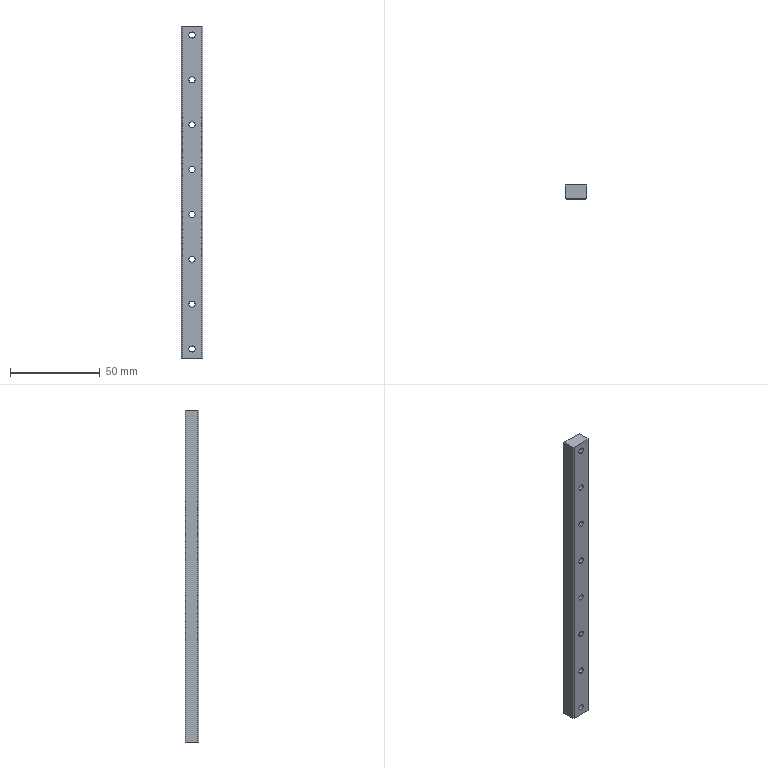Part | SolidWorks | features Chamfer 1, Extrusion 1, HoleWzd 1, LPattern 1 | 1 solid | 48 faces | box 12 x 7.5 x 185 mm | volume 15537 mm3 | cylinder 32 | plane 16 | commonest cylinder face diameters 3.4 x16 6 x16
STEP:
#1=CARTESIAN_POINT('',(0.,-3.75,178.3));
#2=VERTEX_POINT('',#1);
#3=CARTESIAN_POINT('',(0.,-3.75,181.7));
#4=VERTEX_POINT('',#3);
#5=CARTESIAN_POINT('',(0.,-3.75,180.));
#6=DIRECTION('',(0.,1.,0.));
#7=DIRECTION('',(0.,0.,1.));
#8=AXIS2_PLACEMENT_3D('',#5,#6,#7);
#9=CIRCLE('',#8,1.7);
#10=EDGE_CURVE('',#2,#4,#9,.T.);
#11=ORIENTED_EDGE('',*,*,#10,.F.);
#12=CARTESIAN_POINT('',(0.,0.35,178.3));
#13=VERTEX_POINT('',#12);
#14=CARTESIAN_POINT('',(0.,3.75,178.3));
#15=DIRECTION('',(0.,1.,0.));
#16=VECTOR('',#15,1000.);
#17=LINE('',#14,#16);
#18=EDGE_CURVE('',#2,#13,#17,.T.);
#19=ORIENTED_EDGE('',*,*,#18,.T.);
#20=CARTESIAN_POINT('',(0.,0.35,181.7));
#21=VERTEX_POINT('',#20);
#22=CARTESIAN_POINT('',(0.,0.35,180.));
#23=DIRECTION('',(0.,1.,0.));
#24=DIRECTION('',(0.,0.,1.));
#25=AXIS2_PLACEMENT_3D('',#22,#23,#24);
#26=CIRCLE('',#25,1.7);
#27=EDGE_CURVE('',#13,#21,#26,.T.);
#28=ORIENTED_EDGE('',*,*,#27,.T.);
#29=CARTESIAN_POINT('',(0.,3.75,181.7));
#30=DIRECTION('',(0.,1.,0.));
#31=VECTOR('',#30,1000.);
#32=LINE('',#29,#31);
#33=EDGE_CURVE('',#4,#21,#32,.T.);
#34=ORIENTED_EDGE('',*,*,#33,.F.);
#35=EDGE_LOOP('',(#11,#19,#28,#34));
#36=FACE_OUTER_BOUND('',#35,.T.);
#37=CARTESIAN_POINT('',(0.,3.75,180.));
#38=DIRECTION('',(0.,1.,0.));
#39=DIRECTION('',(0.,0.,1.));
#40=AXIS2_PLACEMENT_3D('',#37,#38,#39);
#41=CYLINDRICAL_SURFACE('',#40,1.7);
#42=ADVANCED_FACE('',(#36),#41,.F.);
#43=CARTESIAN_POINT('',(0.,0.35,177.));
#44=VERTEX_POINT('',#43);
#45=CARTESIAN_POINT('',(0.,0.35,183.));
#46=VERTEX_POINT('',#45);
#47=CARTESIAN_POINT('',(0.,0.35,180.));
#48=DIRECTION('',(0.,1.,0.));
#49=DIRECTION('',(0.,0.,1.));
#50=AXIS2_PLACEMENT_3D('',#47,#48,#49);
#51=CIRCLE('',#50,3.);
#52=EDGE_CURVE('',#44,#46,#51,.T.);
#53=ORIENTED_EDGE('',*,*,#52,.F.);
#54=CARTESIAN_POINT('',(0.,3.75,177.));
#55=VERTEX_POINT('',#54);
#56=CARTESIAN_POINT('',(0.,3.75,177.));
#57=DIRECTION('',(0.,1.,0.));
#58=VECTOR('',#57,1000.);
#59=LINE('',#56,#58);
#60=EDGE_CURVE('',#44,#55,#59,.T.);
#61=ORIENTED_EDGE('',*,*,#60,.T.);
#62=CARTESIAN_POINT('',(0.,3.75,183.));
#63=VERTEX_POINT('',#62);
#64=CARTESIAN_POINT('',(0.,3.75,180.));
#65=DIRECTION('',(0.,1.,0.));
#66=DIRECTION('',(0.,0.,1.));
#67=AXIS2_PLACEMENT_3D('',#64,#65,#66);
#68=CIRCLE('',#67,3.);
#69=EDGE_CURVE('',#55,#63,#68,.T.);
#70=ORIENTED_EDGE('',*,*,#69,.T.);
#71=CARTESIAN_POINT('',(0.,3.75,183.));
#72=DIRECTION('',(0.,1.,0.));
#73=VECTOR('',#72,1000.);
#74=LINE('',#71,#73);
#75=EDGE_CURVE('',#46,#63,#74,.T.);
#76=ORIENTED_EDGE('',*,*,#75,.F.);
#77=EDGE_LOOP('',(#53,#61,#70,#76));
#78=FACE_OUTER_BOUND('',#77,.T.);
#79=CARTESIAN_POINT('',(0.,3.75,180.));
#80=DIRECTION('',(0.,1.,0.));
#81=DIRECTION('',(0.,0.,1.));
#82=AXIS2_PLACEMENT_3D('',#79,#80,#81);
#83=CYLINDRICAL_SURFACE('',#82,3.);
#84=ADVANCED_FACE('',(#78),#83,.F.);
#85=CARTESIAN_POINT('',(0.,-3.75,153.3));
#86=VERTEX_POINT('',#85);
#87=CARTESIAN_POINT('',(0.,-3.75,156.7));
#88=VERTEX_POINT('',#87);
#89=CARTESIAN_POINT('',(0.,-3.75,155.));
#90=DIRECTION('',(0.,1.,0.));
#91=DIRECTION('',(0.,0.,1.));
#92=AXIS2_PLACEMENT_3D('',#89,#90,#91);
#93=CIRCLE('',#92,1.7);
#94=EDGE_CURVE('',#86,#88,#93,.T.);
#95=ORIENTED_EDGE('',*,*,#94,.F.);
#96=CARTESIAN_POINT('',(0.,0.35,153.3));
#97=VERTEX_POINT('',#96);
#98=CARTESIAN_POINT('',(0.,3.75,153.3));
#99=DIRECTION('',(0.,1.,0.));
#100=VECTOR('',#99,1000.);
#101=LINE('',#98,#100);
#102=EDGE_CURVE('',#86,#97,#101,.T.);
#103=ORIENTED_EDGE('',*,*,#102,.T.);
#104=CARTESIAN_POINT('',(0.,0.35,156.7));
#105=VERTEX_POINT('',#104);
#106=CARTESIAN_POINT('',(0.,0.35,155.));
#107=DIRECTION('',(0.,1.,0.));
#108=DIRECTION('',(0.,0.,1.));
#109=AXIS2_PLACEMENT_3D('',#106,#107,#108);
#110=CIRCLE('',#109,1.7);
#111=EDGE_CURVE('',#97,#105,#110,.T.);
#112=ORIENTED_EDGE('',*,*,#111,.T.);
#113=CARTESIAN_POINT('',(0.,3.75,156.7));
#114=DIRECTION('',(0.,1.,0.));
#115=VECTOR('',#114,1000.);
#116=LINE('',#113,#115);
#117=EDGE_CURVE('',#88,#105,#116,.T.);
#118=ORIENTED_EDGE('',*,*,#117,.F.);
#119=EDGE_LOOP('',(#95,#103,#112,#118));
#120=FACE_OUTER_BOUND('',#119,.T.);
#121=CARTESIAN_POINT('',(0.,3.75,155.));
#122=DIRECTION('',(0.,1.,0.));
#123=DIRECTION('',(0.,0.,1.));
#124=AXIS2_PLACEMENT_3D('',#121,#122,#123);
#125=CYLINDRICAL_SURFACE('',#124,1.7);
#126=ADVANCED_FACE('',(#120),#125,.F.);
#127=CARTESIAN_POINT('',(0.,0.35,152.));
#128=VERTEX_POINT('',#127);
#129=CARTESIAN_POINT('',(0.,0.35,158.));
#130=VERTEX_POINT('',#129);
#131=CARTESIAN_POINT('',(0.,0.35,155.));
#132=DIRECTION('',(0.,1.,0.));
#133=DIRECTION('',(0.,0.,1.));
#134=AXIS2_PLACEMENT_3D('',#131,#132,#133);
#135=CIRCLE('',#134,3.);
#136=EDGE_CURVE('',#128,#130,#135,.T.);
#137=ORIENTED_EDGE('',*,*,#136,.F.);
#138=CARTESIAN_POINT('',(0.,3.75,152.));
#139=VERTEX_POINT('',#138);
#140=CARTESIAN_POINT('',(0.,3.75,152.));
#141=DIRECTION('',(0.,1.,0.));
#142=VECTOR('',#141,1000.);
#143=LINE('',#140,#142);
#144=EDGE_CURVE('',#128,#139,#143,.T.);
#145=ORIENTED_EDGE('',*,*,#144,.T.);
#146=CARTESIAN_POINT('',(0.,3.75,158.));
#147=VERTEX_POINT('',#146);
#148=CARTESIAN_POINT('',(0.,3.75,155.));
#149=DIRECTION('',(0.,1.,0.));
#150=DIRECTION('',(0.,0.,1.));
#151=AXIS2_PLACEMENT_3D('',#148,#149,#150);
#152=CIRCLE('',#151,3.);
#153=EDGE_CURVE('',#139,#147,#152,.T.);
#154=ORIENTED_EDGE('',*,*,#153,.T.);
#155=CARTESIAN_POINT('',(0.,3.75,158.));
#156=DIRECTION('',(0.,1.,0.));
#157=VECTOR('',#156,1000.);
#158=LINE('',#155,#157);
#159=EDGE_CURVE('',#130,#147,#158,.T.);
#160=ORIENTED_EDGE('',*,*,#159,.F.);
#161=EDGE_LOOP('',(#137,#145,#154,#160));
#162=FACE_OUTER_BOUND('',#161,.T.);
#163=CARTESIAN_POINT('',(0.,3.75,155.));
#164=DIRECTION('',(0.,1.,0.));
#165=DIRECTION('',(0.,0.,1.));
#166=AXIS2_PLACEMENT_3D('',#163,#164,#165);
#167=CYLINDRICAL_SURFACE('',#166,3.);
#168=ADVANCED_FACE('',(#162),#167,.F.);
#169=CARTESIAN_POINT('',(0.,-3.75,128.3));
#170=VERTEX_POINT('',#169);
#171=CARTESIAN_POINT('',(0.,-3.75,131.7));
#172=VERTEX_POINT('',#171);
#173=CARTESIAN_POINT('',(0.,-3.75,130.));
#174=DIRECTION('',(0.,1.,0.));
#175=DIRECTION('',(0.,0.,1.));
#176=AXIS2_PLACEMENT_3D('',#173,#174,#175);
#177=CIRCLE('',#176,1.7);
#178=EDGE_CURVE('',#170,#172,#177,.T.);
#179=ORIENTED_EDGE('',*,*,#178,.F.);
#180=CARTESIAN_POINT('',(0.,0.35,128.3));
#181=VERTEX_POINT('',#180);
#182=CARTESIAN_POINT('',(0.,3.75,128.3));
#183=DIRECTION('',(0.,1.,0.));
#184=VECTOR('',#183,1000.);
#185=LINE('',#182,#184);
#186=EDGE_CURVE('',#170,#181,#185,.T.);
#187=ORIENTED_EDGE('',*,*,#186,.T.);
#188=CARTESIAN_POINT('',(0.,0.35,131.7));
#189=VERTEX_POINT('',#188);
#190=CARTESIAN_POINT('',(0.,0.35,130.));
#191=DIRECTION('',(0.,1.,0.));
#192=DIRECTION('',(0.,0.,1.));
#193=AXIS2_PLACEMENT_3D('',#190,#191,#192);
#194=CIRCLE('',#193,1.7);
#195=EDGE_CURVE('',#181,#189,#194,.T.);
#196=ORIENTED_EDGE('',*,*,#195,.T.);
#197=CARTESIAN_POINT('',(0.,3.75,131.7));
#198=DIRECTION('',(0.,1.,0.));
#199=VECTOR('',#198,1000.);
#200=LINE('',#197,#199);
#201=EDGE_CURVE('',#172,#189,#200,.T.);
#202=ORIENTED_EDGE('',*,*,#201,.F.);
#203=EDGE_LOOP('',(#179,#187,#196,#202));
#204=FACE_OUTER_BOUND('',#203,.T.);
#205=CARTESIAN_POINT('',(0.,3.75,130.));
#206=DIRECTION('',(0.,1.,0.));
#207=DIRECTION('',(0.,0.,1.));
#208=AXIS2_PLACEMENT_3D('',#205,#206,#207);
#209=CYLINDRICAL_SURFACE('',#208,1.7);
#210=ADVANCED_FACE('',(#204),#209,.F.);
#211=CARTESIAN_POINT('',(0.,0.35,127.));
#212=VERTEX_POINT('',#211);
#213=CARTESIAN_POINT('',(0.,0.35,133.));
#214=VERTEX_POINT('',#213);
#215=CARTESIAN_POINT('',(0.,0.35,130.));
#216=DIRECTION('',(0.,1.,0.));
#217=DIRECTION('',(0.,0.,1.));
#218=AXIS2_PLACEMENT_3D('',#215,#216,#217);
#219=CIRCLE('',#218,3.);
#220=EDGE_CURVE('',#212,#214,#219,.T.);
#221=ORIENTED_EDGE('',*,*,#220,.F.);
#222=CARTESIAN_POINT('',(0.,3.75,127.));
#223=VERTEX_POINT('',#222);
#224=CARTESIAN_POINT('',(0.,3.75,127.));
#225=DIRECTION('',(0.,1.,0.));
#226=VECTOR('',#225,1000.);
#227=LINE('',#224,#226);
#228=EDGE_CURVE('',#212,#223,#227,.T.);
#229=ORIENTED_EDGE('',*,*,#228,.T.);
#230=CARTESIAN_POINT('',(0.,3.75,133.));
#231=VERTEX_POINT('',#230);
#232=CARTESIAN_POINT('',(0.,3.75,130.));
#233=DIRECTION('',(0.,1.,0.));
#234=DIRECTION('',(0.,0.,1.));
#235=AXIS2_PLACEMENT_3D('',#232,#233,#234);
#236=CIRCLE('',#235,3.);
#237=EDGE_CURVE('',#223,#231,#236,.T.);
#238=ORIENTED_EDGE('',*,*,#237,.T.);
#239=CARTESIAN_POINT('',(0.,3.75,133.));
#240=DIRECTION('',(0.,1.,0.));
#241=VECTOR('',#240,1000.);
#242=LINE('',#239,#241);
#243=EDGE_CURVE('',#214,#231,#242,.T.);
#244=ORIENTED_EDGE('',*,*,#243,.F.);
#245=EDGE_LOOP('',(#221,#229,#238,#244));
#246=FACE_OUTER_BOUND('',#245,.T.);
#247=CARTESIAN_POINT('',(0.,3.75,130.));
#248=DIRECTION('',(0.,1.,0.));
#249=DIRECTION('',(0.,0.,1.));
#250=AXIS2_PLACEMENT_3D('',#247,#248,#249);
#251=CYLINDRICAL_SURFACE('',#250,3.);
#252=ADVANCED_FACE('',(#246),#251,.F.);
#253=CARTESIAN_POINT('',(0.,-3.75,103.3));
#254=VERTEX_POINT('',#253);
#255=CARTESIAN_POINT('',(0.,-3.75,106.7));
#256=VERTEX_POINT('',#255);
#257=CARTESIAN_POINT('',(0.,-3.75,105.));
#258=DIRECTION('',(0.,1.,0.));
#259=DIRECTION('',(0.,0.,1.));
#260=AXIS2_PLACEMENT_3D('',#257,#258,#259);
#261=CIRCLE('',#260,1.7);
#262=EDGE_CURVE('',#254,#256,#261,.T.);
#263=ORIENTED_EDGE('',*,*,#262,.F.);
#264=CARTESIAN_POINT('',(0.,0.35,103.3));
#265=VERTEX_POINT('',#264);
#266=CARTESIAN_POINT('',(0.,3.75,103.3));
#267=DIRECTION('',(0.,1.,0.));
#268=VECTOR('',#267,1000.);
#269=LINE('',#266,#268);
#270=EDGE_CURVE('',#254,#265,#269,.T.);
#271=ORIENTED_EDGE('',*,*,#270,.T.);
#272=CARTESIAN_POINT('',(0.,0.35,106.7));
#273=VERTEX_POINT('',#272);
#274=CARTESIAN_POINT('',(0.,0.35,105.));
#275=DIRECTION('',(0.,1.,0.));
#276=DIRECTION('',(0.,0.,1.));
#277=AXIS2_PLACEMENT_3D('',#274,#275,#276);
#278=CIRCLE('',#277,1.7);
#279=EDGE_CURVE('',#265,#273,#278,.T.);
#280=ORIENTED_EDGE('',*,*,#279,.T.);
#281=CARTESIAN_POINT('',(0.,3.75,106.7));
#282=DIRECTION('',(0.,1.,0.));
#283=VECTOR('',#282,1000.);
#284=LINE('',#281,#283);
#285=EDGE_CURVE('',#256,#273,#284,.T.);
#286=ORIENTED_EDGE('',*,*,#285,.F.);
#287=EDGE_LOOP('',(#263,#271,#280,#286));
#288=FACE_OUTER_BOUND('',#287,.T.);
#289=CARTESIAN_POINT('',(0.,3.75,105.));
#290=DIRECTION('',(0.,1.,0.));
#291=DIRECTION('',(0.,0.,1.));
#292=AXIS2_PLACEMENT_3D('',#289,#290,#291);
#293=CYLINDRICAL_SURFACE('',#292,1.7);
#294=ADVANCED_FACE('',(#288),#293,.F.);
#295=CARTESIAN_POINT('',(0.,0.35,102.));
#296=VERTEX_POINT('',#295);
#297=CARTESIAN_POINT('',(0.,0.35,108.));
#298=VERTEX_POINT('',#297);
#299=CARTESIAN_POINT('',(0.,0.35,105.));
#300=DIRECTION('',(0.,1.,0.));
#301=DIRECTION('',(0.,0.,1.));
#302=AXIS2_PLACEMENT_3D('',#299,#300,#301);
#303=CIRCLE('',#302,3.);
#304=EDGE_CURVE('',#296,#298,#303,.T.);
#305=ORIENTED_EDGE('',*,*,#304,.F.);
#306=CARTESIAN_POINT('',(0.,3.75,102.));
#307=VERTEX_POINT('',#306);
#308=CARTESIAN_POINT('',(0.,3.75,102.));
#309=DIRECTION('',(0.,1.,0.));
#310=VECTOR('',#309,1000.);
#311=LINE('',#308,#310);
#312=EDGE_CURVE('',#296,#307,#311,.T.);
#313=ORIENTED_EDGE('',*,*,#312,.T.);
#314=CARTESIAN_POINT('',(0.,3.75,108.));
#315=VERTEX_POINT('',#314);
#316=CARTESIAN_POINT('',(0.,3.75,105.));
#317=DIRECTION('',(0.,1.,0.));
#318=DIRECTION('',(0.,0.,1.));
#319=AXIS2_PLACEMENT_3D('',#316,#317,#318);
#320=CIRCLE('',#319,3.);
#321=EDGE_CURVE('',#307,#315,#320,.T.);
#322=ORIENTED_EDGE('',*,*,#321,.T.);
#323=CARTESIAN_POINT('',(0.,3.75,108.));
#324=DIRECTION('',(0.,1.,0.));
#325=VECTOR('',#324,1000.);
#326=LINE('',#323,#325);
#327=EDGE_CURVE('',#298,#315,#326,.T.);
#328=ORIENTED_EDGE('',*,*,#327,.F.);
#329=EDGE_LOOP('',(#305,#313,#322,#328));
#330=FACE_OUTER_BOUND('',#329,.T.);
#331=CARTESIAN_POINT('',(0.,3.75,105.));
#332=DIRECTION('',(0.,1.,0.));
#333=DIRECTION('',(0.,0.,1.));
#334=AXIS2_PLACEMENT_3D('',#331,#332,#333);
#335=CYLINDRICAL_SURFACE('',#334,3.);
#336=ADVANCED_FACE('',(#330),#335,.F.);
#337=CARTESIAN_POINT('',(0.,-3.75,78.3));
#338=VERTEX_POINT('',#337);
#339=CARTESIAN_POINT('',(0.,-3.75,81.7));
#340=VERTEX_POINT('',#339);
#341=CARTESIAN_POINT('',(0.,-3.75,80.));
#342=DIRECTION('',(0.,1.,0.));
#343=DIRECTION('',(0.,0.,1.));
#344=AXIS2_PLACEMENT_3D('',#341,#342,#343);
#345=CIRCLE('',#344,1.7);
#346=EDGE_CURVE('',#338,#340,#345,.T.);
#347=ORIENTED_EDGE('',*,*,#346,.F.);
#348=CARTESIAN_POINT('',(0.,0.35,78.3));
#349=VERTEX_POINT('',#348);
#350=CARTESIAN_POINT('',(0.,3.75,78.3));
#351=DIRECTION('',(0.,1.,0.));
#352=VECTOR('',#351,1000.);
#353=LINE('',#350,#352);
#354=EDGE_CURVE('',#338,#349,#353,.T.);
#355=ORIENTED_EDGE('',*,*,#354,.T.);
#356=CARTESIAN_POINT('',(0.,0.35,81.7));
#357=VERTEX_POINT('',#356);
#358=CARTESIAN_POINT('',(0.,0.35,80.));
#359=DIRECTION('',(0.,1.,0.));
#360=DIRECTION('',(0.,0.,1.));
#361=AXIS2_PLACEMENT_3D('',#358,#359,#360);
#362=CIRCLE('',#361,1.7);
#363=EDGE_CURVE('',#349,#357,#362,.T.);
#364=ORIENTED_EDGE('',*,*,#363,.T.);
#365=CARTESIAN_POINT('',(0.,3.75,81.7));
#366=DIRECTION('',(0.,1.,0.));
#367=VECTOR('',#366,1000.);
#368=LINE('',#365,#367);
#369=EDGE_CURVE('',#340,#357,#368,.T.);
#370=ORIENTED_EDGE('',*,*,#369,.F.);
#371=EDGE_LOOP('',(#347,#355,#364,#370));
#372=FACE_OUTER_BOUND('',#371,.T.);
#373=CARTESIAN_POINT('',(0.,3.75,80.));
#374=DIRECTION('',(0.,1.,0.));
#375=DIRECTION('',(0.,0.,1.));
#376=AXIS2_PLACEMENT_3D('',#373,#374,#375);
#377=CYLINDRICAL_SURFACE('',#376,1.7);
#378=ADVANCED_FACE('',(#372),#377,.F.);
#379=CARTESIAN_POINT('',(0.,0.35,77.));
#380=VERTEX_POINT('',#379);
#381=CARTESIAN_POINT('',(0.,0.35,83.));
#382=VERTEX_POINT('',#381);
#383=CARTESIAN_POINT('',(0.,0.35,80.));
#384=DIRECTION('',(0.,1.,0.));
#385=DIRECTION('',(0.,0.,1.));
#386=AXIS2_PLACEMENT_3D('',#383,#384,#385);
#387=CIRCLE('',#386,3.);
#388=EDGE_CURVE('',#380,#382,#387,.T.);
#389=ORIENTED_EDGE('',*,*,#388,.F.);
#390=CARTESIAN_POINT('',(0.,3.75,77.));
#391=VERTEX_POINT('',#390);
#392=CARTESIAN_POINT('',(0.,3.75,77.));
#393=DIRECTION('',(0.,1.,0.));
#394=VECTOR('',#393,1000.);
#395=LINE('',#392,#394);
#396=EDGE_CURVE('',#380,#391,#395,.T.);
#397=ORIENTED_EDGE('',*,*,#396,.T.);
#398=CARTESIAN_POINT('',(0.,3.75,83.));
#399=VERTEX_POINT('',#398);
#400=CARTESIAN_POINT('',(0.,3.75,80.));
#401=DIRECTION('',(0.,1.,0.));
#402=DIRECTION('',(0.,0.,1.));
#403=AXIS2_PLACEMENT_3D('',#400,#401,#402);
#404=CIRCLE('',#403,3.);
#405=EDGE_CURVE('',#391,#399,#404,.T.);
#406=ORIENTED_EDGE('',*,*,#405,.T.);
#407=CARTESIAN_POINT('',(0.,3.75,83.));
#408=DIRECTION('',(0.,1.,0.));
#409=VECTOR('',#408,1000.);
#410=LINE('',#407,#409);
#411=EDGE_CURVE('',#382,#399,#410,.T.);
#412=ORIENTED_EDGE('',*,*,#411,.F.);
#413=EDGE_LOOP('',(#389,#397,#406,#412));
#414=FACE_OUTER_BOUND('',#413,.T.);
#415=CARTESIAN_POINT('',(0.,3.75,80.));
#416=DIRECTION('',(0.,1.,0.));
#417=DIRECTION('',(0.,0.,1.));
#418=AXIS2_PLACEMENT_3D('',#415,#416,#417);
#419=CYLINDRICAL_SURFACE('',#418,3.);
#420=ADVANCED_FACE('',(#414),#419,.F.);
#421=CARTESIAN_POINT('',(0.,-3.75,53.3));
#422=VERTEX_POINT('',#421);
#423=CARTESIAN_POINT('',(0.,-3.75,56.7));
#424=VERTEX_POINT('',#423);
#425=CARTESIAN_POINT('',(0.,-3.75,55.));
#426=DIRECTION('',(0.,1.,0.));
#427=DIRECTION('',(0.,0.,1.));
#428=AXIS2_PLACEMENT_3D('',#425,#426,#427);
#429=CIRCLE('',#428,1.7);
#430=EDGE_CURVE('',#422,#424,#429,.T.);
#431=ORIENTED_EDGE('',*,*,#430,.F.);
#432=CARTESIAN_POINT('',(0.,0.35,53.3));
#433=VERTEX_POINT('',#432);
#434=CARTESIAN_POINT('',(0.,3.75,53.3));
#435=DIRECTION('',(0.,1.,0.));
#436=VECTOR('',#435,1000.);
#437=LINE('',#434,#436);
#438=EDGE_CURVE('',#422,#433,#437,.T.);
#439=ORIENTED_EDGE('',*,*,#438,.T.);
#440=CARTESIAN_POINT('',(0.,0.35,56.7));
#441=VERTEX_POINT('',#440);
#442=CARTESIAN_POINT('',(0.,0.35,55.));
#443=DIRECTION('',(0.,1.,0.));
#444=DIRECTION('',(0.,0.,1.));
#445=AXIS2_PLACEMENT_3D('',#442,#443,#444);
#446=CIRCLE('',#445,1.7);
#447=EDGE_CURVE('',#433,#441,#446,.T.);
#448=ORIENTED_EDGE('',*,*,#447,.T.);
#449=CARTESIAN_POINT('',(0.,3.75,56.7));
#450=DIRECTION('',(0.,1.,0.));
#451=VECTOR('',#450,1000.);
#452=LINE('',#449,#451);
#453=EDGE_CURVE('',#424,#441,#452,.T.);
#454=ORIENTED_EDGE('',*,*,#453,.F.);
#455=EDGE_LOOP('',(#431,#439,#448,#454));
#456=FACE_OUTER_BOUND('',#455,.T.);
#457=CARTESIAN_POINT('',(0.,3.75,55.));
#458=DIRECTION('',(0.,1.,0.));
#459=DIRECTION('',(0.,0.,1.));
#460=AXIS2_PLACEMENT_3D('',#457,#458,#459);
#461=CYLINDRICAL_SURFACE('',#460,1.7);
#462=ADVANCED_FACE('',(#456),#461,.F.);
#463=CARTESIAN_POINT('',(0.,0.35,52.));
#464=VERTEX_POINT('',#463);
#465=CARTESIAN_POINT('',(0.,0.35,58.));
#466=VERTEX_POINT('',#465);
#467=CARTESIAN_POINT('',(0.,0.35,55.));
#468=DIRECTION('',(0.,1.,0.));
#469=DIRECTION('',(0.,0.,1.));
#470=AXIS2_PLACEMENT_3D('',#467,#468,#469);
#471=CIRCLE('',#470,3.);
#472=EDGE_CURVE('',#464,#466,#471,.T.);
#473=ORIENTED_EDGE('',*,*,#472,.F.);
#474=CARTESIAN_POINT('',(0.,3.75,52.));
#475=VERTEX_POINT('',#474);
#476=CARTESIAN_POINT('',(0.,3.75,52.));
#477=DIRECTION('',(0.,1.,0.));
#478=VECTOR('',#477,1000.);
#479=LINE('',#476,#478);
#480=EDGE_CURVE('',#464,#475,#479,.T.);
#481=ORIENTED_EDGE('',*,*,#480,.T.);
#482=CARTESIAN_POINT('',(0.,3.75,58.));
#483=VERTEX_POINT('',#482);
#484=CARTESIAN_POINT('',(0.,3.75,55.));
#485=DIRECTION('',(0.,1.,0.));
#486=DIRECTION('',(0.,0.,1.));
#487=AXIS2_PLACEMENT_3D('',#484,#485,#486);
#488=CIRCLE('',#487,3.);
#489=EDGE_CURVE('',#475,#483,#488,.T.);
#490=ORIENTED_EDGE('',*,*,#489,.T.);
#491=CARTESIAN_POINT('',(0.,3.75,58.));
#492=DIRECTION('',(0.,1.,0.));
#493=VECTOR('',#492,1000.);
#494=LINE('',#491,#493);
#495=EDGE_CURVE('',#466,#483,#494,.T.);
#496=ORIENTED_EDGE('',*,*,#495,.F.);
#497=EDGE_LOOP('',(#473,#481,#490,#496));
#498=FACE_OUTER_BOUND('',#497,.T.);
#499=CARTESIAN_POINT('',(0.,3.75,55.));
#500=DIRECTION('',(0.,1.,0.));
#501=DIRECTION('',(0.,0.,1.));
#502=AXIS2_PLACEMENT_3D('',#499,#500,#501);
#503=CYLINDRICAL_SURFACE('',#502,3.);
#504=ADVANCED_FACE('',(#498),#503,.F.);
#505=CARTESIAN_POINT('',(0.,0.35,27.));
#506=VERTEX_POINT('',#505);
#507=CARTESIAN_POINT('',(0.,0.35,33.));
#508=VERTEX_POINT('',#507);
#509=CARTESIAN_POINT('',(0.,0.35,30.));
#510=DIRECTION('',(0.,1.,0.));
#511=DIRECTION('',(0.,0.,1.));
#512=AXIS2_PLACEMENT_3D('',#509,#510,#511);
#513=CIRCLE('',#512,3.);
#514=EDGE_CURVE('',#506,#508,#513,.T.);
#515=ORIENTED_EDGE('',*,*,#514,.F.);
#516=CARTESIAN_POINT('',(0.,3.75,27.));
#517=VERTEX_POINT('',#516);
#518=CARTESIAN_POINT('',(0.,3.75,27.));
#519=DIRECTION('',(0.,1.,0.));
#520=VECTOR('',#519,1000.);
#521=LINE('',#518,#520);
#522=EDGE_CURVE('',#506,#517,#521,.T.);
#523=ORIENTED_EDGE('',*,*,#522,.T.);
#524=CARTESIAN_POINT('',(0.,3.75,33.));
#525=VERTEX_POINT('',#524);
#526=CARTESIAN_POINT('',(0.,3.75,30.));
#527=DIRECTION('',(0.,1.,0.));
#528=DIRECTION('',(0.,0.,1.));
#529=AXIS2_PLACEMENT_3D('',#526,#527,#528);
#530=CIRCLE('',#529,3.);
#531=EDGE_CURVE('',#517,#525,#530,.T.);
#532=ORIENTED_EDGE('',*,*,#531,.T.);
#533=CARTESIAN_POINT('',(0.,3.75,33.));
#534=DIRECTION('',(0.,1.,0.));
#535=VECTOR('',#534,1000.);
#536=LINE('',#533,#535);
#537=EDGE_CURVE('',#508,#525,#536,.T.);
#538=ORIENTED_EDGE('',*,*,#537,.F.);
#539=EDGE_LOOP('',(#515,#523,#532,#538));
#540=FACE_OUTER_BOUND('',#539,.T.);
#541=CARTESIAN_POINT('',(0.,3.75,30.));
#542=DIRECTION('',(0.,1.,0.));
#543=DIRECTION('',(0.,0.,1.));
#544=AXIS2_PLACEMENT_3D('',#541,#542,#543);
#545=CYLINDRICAL_SURFACE('',#544,3.);
#546=ADVANCED_FACE('',(#540),#545,.F.);
#547=CARTESIAN_POINT('',(0.,-3.75,28.3));
#548=VERTEX_POINT('',#547);
#549=CARTESIAN_POINT('',(0.,-3.75,31.7));
#550=VERTEX_POINT('',#549);
#551=CARTESIAN_POINT('',(0.,-3.75,30.));
#552=DIRECTION('',(0.,1.,0.));
#553=DIRECTION('',(0.,0.,1.));
#554=AXIS2_PLACEMENT_3D('',#551,#552,#553);
#555=CIRCLE('',#554,1.7);
#556=EDGE_CURVE('',#548,#550,#555,.T.);
#557=ORIENTED_EDGE('',*,*,#556,.F.);
#558=CARTESIAN_POINT('',(0.,0.35,28.3));
#559=VERTEX_POINT('',#558);
#560=CARTESIAN_POINT('',(0.,3.75,28.3));
#561=DIRECTION('',(0.,1.,0.));
#562=VECTOR('',#561,1000.);
#563=LINE('',#560,#562);
#564=EDGE_CURVE('',#548,#559,#563,.T.);
#565=ORIENTED_EDGE('',*,*,#564,.T.);
#566=CARTESIAN_POINT('',(0.,0.35,31.7));
#567=VERTEX_POINT('',#566);
#568=CARTESIAN_POINT('',(0.,0.35,30.));
#569=DIRECTION('',(0.,1.,0.));
#570=DIRECTION('',(0.,0.,1.));
#571=AXIS2_PLACEMENT_3D('',#568,#569,#570);
#572=CIRCLE('',#571,1.7);
#573=EDGE_CURVE('',#559,#567,#572,.T.);
#574=ORIENTED_EDGE('',*,*,#573,.T.);
#575=CARTESIAN_POINT('',(0.,3.75,31.7));
#576=DIRECTION('',(0.,1.,0.));
#577=VECTOR('',#576,1000.);
#578=LINE('',#575,#577);
#579=EDGE_CURVE('',#550,#567,#578,.T.);
#580=ORIENTED_EDGE('',*,*,#579,.F.);
#581=EDGE_LOOP('',(#557,#565,#574,#580));
#582=FACE_OUTER_BOUND('',#581,.T.);
#583=CARTESIAN_POINT('',(0.,3.75,30.));
#584=DIRECTION('',(0.,1.,0.));
#585=DIRECTION('',(0.,0.,1.));
#586=AXIS2_PLACEMENT_3D('',#583,#584,#585);
#587=CYLINDRICAL_SURFACE('',#586,1.7);
#588=ADVANCED_FACE('',(#582),#587,.F.);
#589=CARTESIAN_POINT('',(0.,0.35,2.));
#590=VERTEX_POINT('',#589);
#591=CARTESIAN_POINT('',(0.,0.35,8.));
#592=VERTEX_POINT('',#591);
#593=CARTESIAN_POINT('',(0.,0.35,5.));
#594=DIRECTION('',(0.,1.,0.));
#595=DIRECTION('',(0.,0.,1.));
#596=AXIS2_PLACEMENT_3D('',#593,#594,#595);
#597=CIRCLE('',#596,3.);
#598=EDGE_CURVE('',#590,#592,#597,.T.);
#599=ORIENTED_EDGE('',*,*,#598,.F.);
#600=CARTESIAN_POINT('',(0.,3.75,2.));
#601=VERTEX_POINT('',#600);
#602=CARTESIAN_POINT('',(0.,3.75,2.));
#603=DIRECTION('',(0.,1.,0.));
#604=VECTOR('',#603,1000.);
#605=LINE('',#602,#604);
#606=EDGE_CURVE('',#590,#601,#605,.T.);
#607=ORIENTED_EDGE('',*,*,#606,.T.);
#608=CARTESIAN_POINT('',(0.,3.75,8.));
#609=VERTEX_POINT('',#608);
#610=CARTESIAN_POINT('',(0.,3.75,5.));
#611=DIRECTION('',(0.,1.,0.));
#612=DIRECTION('',(0.,0.,1.));
#613=AXIS2_PLACEMENT_3D('',#610,#611,#612);
#614=CIRCLE('',#613,3.);
#615=EDGE_CURVE('',#601,#609,#614,.T.);
#616=ORIENTED_EDGE('',*,*,#615,.T.);
#617=CARTESIAN_POINT('',(0.,3.75,8.));
#618=DIRECTION('',(0.,1.,0.));
#619=VECTOR('',#618,1000.);
#620=LINE('',#617,#619);
#621=EDGE_CURVE('',#592,#609,#620,.T.);
#622=ORIENTED_EDGE('',*,*,#621,.F.);
#623=EDGE_LOOP('',(#599,#607,#616,#622));
#624=FACE_OUTER_BOUND('',#623,.T.);
#625=CARTESIAN_POINT('',(0.,3.75,5.));
#626=DIRECTION('',(0.,1.,0.));
#627=DIRECTION('',(0.,0.,1.));
#628=AXIS2_PLACEMENT_3D('',#625,#626,#627);
#629=CYLINDRICAL_SURFACE('',#628,3.);
#630=ADVANCED_FACE('',(#624),#629,.F.);
#631=CARTESIAN_POINT('',(0.,-3.75,3.3));
#632=VERTEX_POINT('',#631);
#633=CARTESIAN_POINT('',(0.,-3.75,6.7));
#634=VERTEX_POINT('',#633);
#635=CARTESIAN_POINT('',(0.,-3.75,5.));
#636=DIRECTION('',(0.,1.,0.));
#637=DIRECTION('',(0.,0.,1.));
#638=AXIS2_PLACEMENT_3D('',#635,#636,#637);
#639=CIRCLE('',#638,1.7);
#640=EDGE_CURVE('',#632,#634,#639,.T.);
#641=ORIENTED_EDGE('',*,*,#640,.F.);
#642=CARTESIAN_POINT('',(0.,0.35,3.3));
#643=VERTEX_POINT('',#642);
#644=CARTESIAN_POINT('',(0.,3.75,3.3));
#645=DIRECTION('',(0.,1.,0.));
#646=VECTOR('',#645,1000.);
#647=LINE('',#644,#646);
#648=EDGE_CURVE('',#632,#643,#647,.T.);
#649=ORIENTED_EDGE('',*,*,#648,.T.);
#650=CARTESIAN_POINT('',(0.,0.35,6.7));
#651=VERTEX_POINT('',#650);
#652=CARTESIAN_POINT('',(0.,0.35,5.));
#653=DIRECTION('',(0.,1.,0.));
#654=DIRECTION('',(0.,0.,1.));
#655=AXIS2_PLACEMENT_3D('',#652,#653,#654);
#656=CIRCLE('',#655,1.7);
#657=EDGE_CURVE('',#643,#651,#656,.T.);
#658=ORIENTED_EDGE('',*,*,#657,.T.);
#659=CARTESIAN_POINT('',(0.,3.75,6.7));
#660=DIRECTION('',(0.,1.,0.));
#661=VECTOR('',#660,1000.);
#662=LINE('',#659,#661);
#663=EDGE_CURVE('',#634,#651,#662,.T.);
#664=ORIENTED_EDGE('',*,*,#663,.F.);
#665=EDGE_LOOP('',(#641,#649,#658,#664));
#666=FACE_OUTER_BOUND('',#665,.T.);
#667=CARTESIAN_POINT('',(0.,3.75,5.));
#668=DIRECTION('',(0.,1.,0.));
#669=DIRECTION('',(0.,0.,1.));
#670=AXIS2_PLACEMENT_3D('',#667,#668,#669);
#671=CYLINDRICAL_SURFACE('',#670,1.7);
#672=ADVANCED_FACE('',(#666),#671,.F.);
#673=CARTESIAN_POINT('',(6.,-3.25,185.));
#674=VERTEX_POINT('',#673);
#675=CARTESIAN_POINT('',(6.,3.75,185.));
#676=VERTEX_POINT('',#675);
#677=CARTESIAN_POINT('',(6.,3.75,185.));
#678=DIRECTION('',(0.,1.,0.));
#679=VECTOR('',#678,1000.);
#680=LINE('',#677,#679);
#681=EDGE_CURVE('',#674,#676,#680,.T.);
#682=ORIENTED_EDGE('',*,*,#681,.F.);
#683=CARTESIAN_POINT('',(6.,-3.25,0.));
#684=VERTEX_POINT('',#683);
#685=CARTESIAN_POINT('',(6.,-3.25,185.));
#686=DIRECTION('',(0.,0.,-1.));
#687=VECTOR('',#686,1000.);
#688=LINE('',#685,#687);
#689=EDGE_CURVE('',#674,#684,#688,.T.);
#690=ORIENTED_EDGE('',*,*,#689,.T.);
#691=CARTESIAN_POINT('',(6.,3.75,0.));
#692=VERTEX_POINT('',#691);
#693=CARTESIAN_POINT('',(6.,3.75,0.));
#694=DIRECTION('',(0.,1.,0.));
#695=VECTOR('',#694,1000.);
#696=LINE('',#693,#695);
#697=EDGE_CURVE('',#684,#692,#696,.T.);
#698=ORIENTED_EDGE('',*,*,#697,.T.);
#699=CARTESIAN_POINT('',(6.,3.75,185.));
#700=DIRECTION('',(0.,0.,-1.));
#701=VECTOR('',#700,1000.);
#702=LINE('',#699,#701);
#703=EDGE_CURVE('',#676,#692,#702,.T.);
#704=ORIENTED_EDGE('',*,*,#703,.F.);
#705=EDGE_LOOP('',(#682,#690,#698,#704));
#706=FACE_OUTER_BOUND('',#705,.T.);
#707=CARTESIAN_POINT('',(6.,3.75,185.));
#708=DIRECTION('',(-1.,0.,0.));
#709=DIRECTION('',(0.,-1.,0.));
#710=AXIS2_PLACEMENT_3D('',#707,#708,#709);
#711=PLANE('',#710);
#712=ADVANCED_FACE('',(#706),#711,.F.);
#713=CARTESIAN_POINT('',(0.,3.75,30.));
#714=DIRECTION('',(0.,1.,0.));
#715=DIRECTION('',(0.,0.,1.));
#716=AXIS2_PLACEMENT_3D('',#713,#714,#715);
#717=CIRCLE('',#716,3.);
#718=EDGE_CURVE('',#525,#517,#717,.T.);
#719=ORIENTED_EDGE('',*,*,#718,.F.);
#720=ORIENTED_EDGE('',*,*,#531,.F.);
#721=EDGE_LOOP('',(#719,#720));
#722=FACE_BOUND('',#721,.T.);
#723=CARTESIAN_POINT('',(0.,3.75,5.));
#724=DIRECTION('',(0.,1.,0.));
#725=DIRECTION('',(0.,0.,1.));
#726=AXIS2_PLACEMENT_3D('',#723,#724,#725);
#727=CIRCLE('',#726,3.);
#728=EDGE_CURVE('',#609,#601,#727,.T.);
#729=ORIENTED_EDGE('',*,*,#728,.F.);
#730=ORIENTED_EDGE('',*,*,#615,.F.);
#731=EDGE_LOOP('',(#729,#730));
#732=FACE_BOUND('',#731,.T.);
#733=CARTESIAN_POINT('',(-6.,3.75,0.));
#734=VERTEX_POINT('',#733);
#735=CARTESIAN_POINT('',(-6.,3.75,0.));
#736=DIRECTION('',(-1.,0.,0.));
#737=VECTOR('',#736,1000.);
#738=LINE('',#735,#737);
#739=EDGE_CURVE('',#692,#734,#738,.T.);
#740=ORIENTED_EDGE('',*,*,#739,.T.);
#741=CARTESIAN_POINT('',(-6.,3.75,185.));
#742=VERTEX_POINT('',#741);
#743=CARTESIAN_POINT('',(-6.,3.75,185.));
#744=DIRECTION('',(0.,0.,-1.));
#745=VECTOR('',#744,1000.);
#746=LINE('',#743,#745);
#747=EDGE_CURVE('',#742,#734,#746,.T.);
#748=ORIENTED_EDGE('',*,*,#747,.F.);
#749=CARTESIAN_POINT('',(-6.,3.75,185.));
#750=DIRECTION('',(-1.,0.,0.));
#751=VECTOR('',#750,1000.);
#752=LINE('',#749,#751);
#753=EDGE_CURVE('',#676,#742,#752,.T.);
#754=ORIENTED_EDGE('',*,*,#753,.F.);
#755=ORIENTED_EDGE('',*,*,#703,.T.);
#756=EDGE_LOOP('',(#740,#748,#754,#755));
#757=FACE_OUTER_BOUND('',#756,.T.);
#758=CARTESIAN_POINT('',(0.,3.75,55.));
#759=DIRECTION('',(0.,1.,0.));
#760=DIRECTION('',(0.,0.,1.));
#761=AXIS2_PLACEMENT_3D('',#758,#759,#760);
#762=CIRCLE('',#761,3.);
#763=EDGE_CURVE('',#483,#475,#762,.T.);
#764=ORIENTED_EDGE('',*,*,#763,.F.);
#765=ORIENTED_EDGE('',*,*,#489,.F.);
#766=EDGE_LOOP('',(#764,#765));
#767=FACE_BOUND('',#766,.T.);
#768=CARTESIAN_POINT('',(0.,3.75,80.));
#769=DIRECTION('',(0.,1.,0.));
#770=DIRECTION('',(0.,0.,1.));
#771=AXIS2_PLACEMENT_3D('',#768,#769,#770);
#772=CIRCLE('',#771,3.);
#773=EDGE_CURVE('',#399,#391,#772,.T.);
#774=ORIENTED_EDGE('',*,*,#773,.F.);
#775=ORIENTED_EDGE('',*,*,#405,.F.);
#776=EDGE_LOOP('',(#774,#775));
#777=FACE_BOUND('',#776,.T.);
#778=CARTESIAN_POINT('',(0.,3.75,105.));
#779=DIRECTION('',(0.,1.,0.));
#780=DIRECTION('',(0.,0.,1.));
#781=AXIS2_PLACEMENT_3D('',#778,#779,#780);
#782=CIRCLE('',#781,3.);
#783=EDGE_CURVE('',#315,#307,#782,.T.);
#784=ORIENTED_EDGE('',*,*,#783,.F.);
#785=ORIENTED_EDGE('',*,*,#321,.F.);
#786=EDGE_LOOP('',(#784,#785));
#787=FACE_BOUND('',#786,.T.);
#788=CARTESIAN_POINT('',(0.,3.75,130.));
#789=DIRECTION('',(0.,1.,0.));
#790=DIRECTION('',(0.,0.,1.));
#791=AXIS2_PLACEMENT_3D('',#788,#789,#790);
#792=CIRCLE('',#791,3.);
#793=EDGE_CURVE('',#231,#223,#792,.T.);
#794=ORIENTED_EDGE('',*,*,#793,.F.);
#795=ORIENTED_EDGE('',*,*,#237,.F.);
#796=EDGE_LOOP('',(#794,#795));
#797=FACE_BOUND('',#796,.T.);
#798=CARTESIAN_POINT('',(0.,3.75,155.));
#799=DIRECTION('',(0.,1.,0.));
#800=DIRECTION('',(0.,0.,1.));
#801=AXIS2_PLACEMENT_3D('',#798,#799,#800);
#802=CIRCLE('',#801,3.);
#803=EDGE_CURVE('',#147,#139,#802,.T.);
#804=ORIENTED_EDGE('',*,*,#803,.F.);
#805=ORIENTED_EDGE('',*,*,#153,.F.);
#806=EDGE_LOOP('',(#804,#805));
#807=FACE_BOUND('',#806,.T.);
#808=CARTESIAN_POINT('',(0.,3.75,180.));
#809=DIRECTION('',(0.,1.,0.));
#810=DIRECTION('',(0.,0.,1.));
#811=AXIS2_PLACEMENT_3D('',#808,#809,#810);
#812=CIRCLE('',#811,3.);
#813=EDGE_CURVE('',#63,#55,#812,.T.);
#814=ORIENTED_EDGE('',*,*,#813,.F.);
#815=ORIENTED_EDGE('',*,*,#69,.F.);
#816=EDGE_LOOP('',(#814,#815));
#817=FACE_BOUND('',#816,.T.);
#818=CARTESIAN_POINT('',(-6.,3.75,185.));
#819=DIRECTION('',(0.,-1.,0.));
#820=DIRECTION('',(0.,0.,-1.));
#821=AXIS2_PLACEMENT_3D('',#818,#819,#820);
#822=PLANE('',#821);
#823=ADVANCED_FACE('',(#722,#732,#757,#767,#777,#787,#797,#807,#817),#822,.F.);
#824=CARTESIAN_POINT('',(-6.,-3.25,0.));
#825=VERTEX_POINT('',#824);
#826=CARTESIAN_POINT('',(-6.,3.75,0.));
#827=DIRECTION('',(0.,-1.,0.));
#828=VECTOR('',#827,1000.);
#829=LINE('',#826,#828);
#830=EDGE_CURVE('',#734,#825,#829,.T.);
#831=ORIENTED_EDGE('',*,*,#830,.T.);
#832=CARTESIAN_POINT('',(-6.,-3.25,185.));
#833=VERTEX_POINT('',#832);
#834=CARTESIAN_POINT('',(-6.,-3.25,185.));
#835=DIRECTION('',(0.,0.,1.));
#836=VECTOR('',#835,1000.);
#837=LINE('',#834,#836);
#838=EDGE_CURVE('',#825,#833,#837,.T.);
#839=ORIENTED_EDGE('',*,*,#838,.T.);
#840=CARTESIAN_POINT('',(-6.,3.75,185.));
#841=DIRECTION('',(0.,-1.,0.));
#842=VECTOR('',#841,1000.);
#843=LINE('',#840,#842);
#844=EDGE_CURVE('',#742,#833,#843,.T.);
#845=ORIENTED_EDGE('',*,*,#844,.F.);
#846=ORIENTED_EDGE('',*,*,#747,.T.);
#847=EDGE_LOOP('',(#831,#839,#845,#846));
#848=FACE_OUTER_BOUND('',#847,.T.);
#849=CARTESIAN_POINT('',(-6.,3.75,185.));
#850=DIRECTION('',(1.,0.,0.));
#851=DIRECTION('',(0.,1.,0.));
#852=AXIS2_PLACEMENT_3D('',#849,#850,#851);
#853=PLANE('',#852);
#854=ADVANCED_FACE('',(#848),#853,.F.);
#855=CARTESIAN_POINT('',(0.,-3.75,30.));
#856=DIRECTION('',(0.,1.,0.));
#857=DIRECTION('',(0.,0.,1.));
#858=AXIS2_PLACEMENT_3D('',#855,#856,#857);
#859=CIRCLE('',#858,1.7);
#860=EDGE_CURVE('',#550,#548,#859,.T.);
#861=ORIENTED_EDGE('',*,*,#860,.T.);
#862=ORIENTED_EDGE('',*,*,#556,.T.);
#863=EDGE_LOOP('',(#861,#862));
#864=FACE_BOUND('',#863,.T.);
#865=CARTESIAN_POINT('',(0.,-3.75,5.));
#866=DIRECTION('',(0.,1.,0.));
#867=DIRECTION('',(0.,0.,1.));
#868=AXIS2_PLACEMENT_3D('',#865,#866,#867);
#869=CIRCLE('',#868,1.7);
#870=EDGE_CURVE('',#634,#632,#869,.T.);
#871=ORIENTED_EDGE('',*,*,#870,.T.);
#872=ORIENTED_EDGE('',*,*,#640,.T.);
#873=EDGE_LOOP('',(#871,#872));
#874=FACE_BOUND('',#873,.T.);
#875=CARTESIAN_POINT('',(-5.5,-3.75,0.));
#876=VERTEX_POINT('',#875);
#877=CARTESIAN_POINT('',(5.5,-3.75,0.));
#878=VERTEX_POINT('',#877);
#879=CARTESIAN_POINT('',(-6.,-3.75,0.));
#880=DIRECTION('',(1.,0.,0.));
#881=VECTOR('',#880,1000.);
#882=LINE('',#879,#881);
#883=EDGE_CURVE('',#876,#878,#882,.T.);
#884=ORIENTED_EDGE('',*,*,#883,.T.);
#885=CARTESIAN_POINT('',(5.5,-3.75,185.));
#886=VERTEX_POINT('',#885);
#887=CARTESIAN_POINT('',(5.5,-3.75,185.));
#888=DIRECTION('',(0.,0.,1.));
#889=VECTOR('',#888,1000.);
#890=LINE('',#887,#889);
#891=EDGE_CURVE('',#878,#886,#890,.T.);
#892=ORIENTED_EDGE('',*,*,#891,.T.);
#893=CARTESIAN_POINT('',(-5.5,-3.75,185.));
#894=VERTEX_POINT('',#893);
#895=CARTESIAN_POINT('',(-6.,-3.75,185.));
#896=DIRECTION('',(1.,0.,0.));
#897=VECTOR('',#896,1000.);
#898=LINE('',#895,#897);
#899=EDGE_CURVE('',#894,#886,#898,.T.);
#900=ORIENTED_EDGE('',*,*,#899,.F.);
#901=CARTESIAN_POINT('',(-5.5,-3.75,185.));
#902=DIRECTION('',(0.,0.,-1.));
#903=VECTOR('',#902,1000.);
#904=LINE('',#901,#903);
#905=EDGE_CURVE('',#894,#876,#904,.T.);
#906=ORIENTED_EDGE('',*,*,#905,.T.);
#907=EDGE_LOOP('',(#884,#892,#900,#906));
#908=FACE_OUTER_BOUND('',#907,.T.);
#909=CARTESIAN_POINT('',(0.,-3.75,55.));
#910=DIRECTION('',(0.,1.,0.));
#911=DIRECTION('',(0.,0.,1.));
#912=AXIS2_PLACEMENT_3D('',#909,#910,#911);
#913=CIRCLE('',#912,1.7);
#914=EDGE_CURVE('',#424,#422,#913,.T.);
#915=ORIENTED_EDGE('',*,*,#914,.T.);
#916=ORIENTED_EDGE('',*,*,#430,.T.);
#917=EDGE_LOOP('',(#915,#916));
#918=FACE_BOUND('',#917,.T.);
#919=CARTESIAN_POINT('',(0.,-3.75,80.));
#920=DIRECTION('',(0.,1.,0.));
#921=DIRECTION('',(0.,0.,1.));
#922=AXIS2_PLACEMENT_3D('',#919,#920,#921);
#923=CIRCLE('',#922,1.7);
#924=EDGE_CURVE('',#340,#338,#923,.T.);
#925=ORIENTED_EDGE('',*,*,#924,.T.);
#926=ORIENTED_EDGE('',*,*,#346,.T.);
#927=EDGE_LOOP('',(#925,#926));
#928=FACE_BOUND('',#927,.T.);
#929=CARTESIAN_POINT('',(0.,-3.75,105.));
#930=DIRECTION('',(0.,1.,0.));
#931=DIRECTION('',(0.,0.,1.));
#932=AXIS2_PLACEMENT_3D('',#929,#930,#931);
#933=CIRCLE('',#932,1.7);
#934=EDGE_CURVE('',#256,#254,#933,.T.);
#935=ORIENTED_EDGE('',*,*,#934,.T.);
#936=ORIENTED_EDGE('',*,*,#262,.T.);
#937=EDGE_LOOP('',(#935,#936));
#938=FACE_BOUND('',#937,.T.);
#939=CARTESIAN_POINT('',(0.,-3.75,130.));
#940=DIRECTION('',(0.,1.,0.));
#941=DIRECTION('',(0.,0.,1.));
#942=AXIS2_PLACEMENT_3D('',#939,#940,#941);
#943=CIRCLE('',#942,1.7);
#944=EDGE_CURVE('',#172,#170,#943,.T.);
#945=ORIENTED_EDGE('',*,*,#944,.T.);
#946=ORIENTED_EDGE('',*,*,#178,.T.);
#947=EDGE_LOOP('',(#945,#946));
#948=FACE_BOUND('',#947,.T.);
#949=CARTESIAN_POINT('',(0.,-3.75,155.));
#950=DIRECTION('',(0.,1.,0.));
#951=DIRECTION('',(0.,0.,1.));
#952=AXIS2_PLACEMENT_3D('',#949,#950,#951);
#953=CIRCLE('',#952,1.7);
#954=EDGE_CURVE('',#88,#86,#953,.T.);
#955=ORIENTED_EDGE('',*,*,#954,.T.);
#956=ORIENTED_EDGE('',*,*,#94,.T.);
#957=EDGE_LOOP('',(#955,#956));
#958=FACE_BOUND('',#957,.T.);
#959=CARTESIAN_POINT('',(0.,-3.75,180.));
#960=DIRECTION('',(0.,1.,0.));
#961=DIRECTION('',(0.,0.,1.));
#962=AXIS2_PLACEMENT_3D('',#959,#960,#961);
#963=CIRCLE('',#962,1.7);
#964=EDGE_CURVE('',#4,#2,#963,.T.);
#965=ORIENTED_EDGE('',*,*,#964,.T.);
#966=ORIENTED_EDGE('',*,*,#10,.T.);
#967=EDGE_LOOP('',(#965,#966));
#968=FACE_BOUND('',#967,.T.);
#969=CARTESIAN_POINT('',(-6.,-3.75,185.));
#970=DIRECTION('',(0.,1.,0.));
#971=DIRECTION('',(0.,0.,1.));
#972=AXIS2_PLACEMENT_3D('',#969,#970,#971);
#973=PLANE('',#972);
#974=ADVANCED_FACE('',(#864,#874,#908,#918,#928,#938,#948,#958,#968),#973,.F.);
#975=ORIENTED_EDGE('',*,*,#899,.T.);
#976=CARTESIAN_POINT('',(5.75,-3.5,185.));
#977=DIRECTION('',(0.7071,0.7071,0.));
#978=VECTOR('',#977,1000.);
#979=LINE('',#976,#978);
#980=EDGE_CURVE('',#886,#674,#979,.T.);
#981=ORIENTED_EDGE('',*,*,#980,.T.);
#982=ORIENTED_EDGE('',*,*,#681,.T.);
#983=ORIENTED_EDGE('',*,*,#753,.T.);
#984=ORIENTED_EDGE('',*,*,#844,.T.);
#985=CARTESIAN_POINT('',(0.25,-9.5,185.));
#986=DIRECTION('',(0.7071,-0.7071,0.));
#987=VECTOR('',#986,1000.);
#988=LINE('',#985,#987);
#989=EDGE_CURVE('',#833,#894,#988,.T.);
#990=ORIENTED_EDGE('',*,*,#989,.T.);
#991=EDGE_LOOP('',(#975,#981,#982,#983,#984,#990));
#992=FACE_OUTER_BOUND('',#991,.T.);
#993=CARTESIAN_POINT('',(6.,-3.75,185.));
#994=DIRECTION('',(0.,0.,1.));
#995=DIRECTION('',(1.,0.,0.));
#996=AXIS2_PLACEMENT_3D('',#993,#994,#995);
#997=PLANE('',#996);
#998=ADVANCED_FACE('',(#992),#997,.T.);
#999=ORIENTED_EDGE('',*,*,#697,.F.);
#1000=CARTESIAN_POINT('',(6.,-3.25,0.));
#1001=DIRECTION('',(-0.7071,-0.7071,0.));
#1002=VECTOR('',#1001,1000.);
#1003=LINE('',#1000,#1002);
#1004=EDGE_CURVE('',#684,#878,#1003,.T.);
#1005=ORIENTED_EDGE('',*,*,#1004,.T.);
#1006=ORIENTED_EDGE('',*,*,#883,.F.);
#1007=CARTESIAN_POINT('',(-5.5,-3.75,0.));
#1008=DIRECTION('',(-0.7071,0.7071,0.));
#1009=VECTOR('',#1008,1000.);
#1010=LINE('',#1007,#1009);
#1011=EDGE_CURVE('',#876,#825,#1010,.T.);
#1012=ORIENTED_EDGE('',*,*,#1011,.T.);
#1013=ORIENTED_EDGE('',*,*,#830,.F.);
#1014=ORIENTED_EDGE('',*,*,#739,.F.);
#1015=EDGE_LOOP('',(#999,#1005,#1006,#1012,#1013,#1014));
#1016=FACE_OUTER_BOUND('',#1015,.T.);
#1017=CARTESIAN_POINT('',(6.,-3.75,0.));
#1018=DIRECTION('',(0.,0.,1.));
#1019=DIRECTION('',(1.,0.,0.));
#1020=AXIS2_PLACEMENT_3D('',#1017,#1018,#1019);
#1021=PLANE('',#1020);
#1022=ADVANCED_FACE('',(#1016),#1021,.F.);
#1023=ORIENTED_EDGE('',*,*,#980,.F.);
#1024=ORIENTED_EDGE('',*,*,#891,.F.);
#1025=ORIENTED_EDGE('',*,*,#1004,.F.);
#1026=ORIENTED_EDGE('',*,*,#689,.F.);
#1027=EDGE_LOOP('',(#1023,#1024,#1025,#1026));
#1028=FACE_OUTER_BOUND('',#1027,.T.);
#1029=CARTESIAN_POINT('',(6.,-3.25,185.));
#1030=DIRECTION('',(-0.7071,0.7071,0.));
#1031=DIRECTION('',(-0.7071,-0.7071,0.));
#1032=AXIS2_PLACEMENT_3D('',#1029,#1030,#1031);
#1033=PLANE('',#1032);
#1034=ADVANCED_FACE('',(#1028),#1033,.F.);
#1035=ORIENTED_EDGE('',*,*,#989,.F.);
#1036=ORIENTED_EDGE('',*,*,#838,.F.);
#1037=ORIENTED_EDGE('',*,*,#1011,.F.);
#1038=ORIENTED_EDGE('',*,*,#905,.F.);
#1039=EDGE_LOOP('',(#1035,#1036,#1037,#1038));
#1040=FACE_OUTER_BOUND('',#1039,.T.);
#1041=CARTESIAN_POINT('',(-5.5,-3.75,185.));
#1042=DIRECTION('',(0.7071,0.7071,0.));
#1043=DIRECTION('',(-0.7071,0.7071,0.));
#1044=AXIS2_PLACEMENT_3D('',#1041,#1042,#1043);
#1045=PLANE('',#1044);
#1046=ADVANCED_FACE('',(#1040),#1045,.F.);
#1047=ORIENTED_EDGE('',*,*,#648,.F.);
#1048=ORIENTED_EDGE('',*,*,#870,.F.);
#1049=ORIENTED_EDGE('',*,*,#663,.T.);
#1050=CARTESIAN_POINT('',(0.,0.35,5.));
#1051=DIRECTION('',(0.,1.,0.));
#1052=DIRECTION('',(0.,0.,1.));
#1053=AXIS2_PLACEMENT_3D('',#1050,#1051,#1052);
#1054=CIRCLE('',#1053,1.7);
#1055=EDGE_CURVE('',#651,#643,#1054,.T.);
#1056=ORIENTED_EDGE('',*,*,#1055,.T.);
#1057=EDGE_LOOP('',(#1047,#1048,#1049,#1056));
#1058=FACE_OUTER_BOUND('',#1057,.T.);
#1059=CARTESIAN_POINT('',(0.,3.75,5.));
#1060=DIRECTION('',(0.,1.,0.));
#1061=DIRECTION('',(0.,0.,1.));
#1062=AXIS2_PLACEMENT_3D('',#1059,#1060,#1061);
#1063=CYLINDRICAL_SURFACE('',#1062,1.7);
#1064=ADVANCED_FACE('',(#1058),#1063,.F.);
#1065=ORIENTED_EDGE('',*,*,#1055,.F.);
#1066=ORIENTED_EDGE('',*,*,#657,.F.);
#1067=EDGE_LOOP('',(#1065,#1066));
#1068=FACE_BOUND('',#1067,.T.);
#1069=CARTESIAN_POINT('',(0.,0.35,5.));
#1070=DIRECTION('',(0.,1.,0.));
#1071=DIRECTION('',(0.,0.,1.));
#1072=AXIS2_PLACEMENT_3D('',#1069,#1070,#1071);
#1073=CIRCLE('',#1072,3.);
#1074=EDGE_CURVE('',#592,#590,#1073,.T.);
#1075=ORIENTED_EDGE('',*,*,#1074,.T.);
#1076=ORIENTED_EDGE('',*,*,#598,.T.);
#1077=EDGE_LOOP('',(#1075,#1076));
#1078=FACE_OUTER_BOUND('',#1077,.T.);
#1079=CARTESIAN_POINT('',(1.7,0.35,5.));
#1080=DIRECTION('',(0.,-1.,0.));
#1081=DIRECTION('',(0.,0.,-1.));
#1082=AXIS2_PLACEMENT_3D('',#1079,#1080,#1081);
#1083=PLANE('',#1082);
#1084=ADVANCED_FACE('',(#1068,#1078),#1083,.F.);
#1085=ORIENTED_EDGE('',*,*,#606,.F.);
#1086=ORIENTED_EDGE('',*,*,#1074,.F.);
#1087=ORIENTED_EDGE('',*,*,#621,.T.);
#1088=ORIENTED_EDGE('',*,*,#728,.T.);
#1089=EDGE_LOOP('',(#1085,#1086,#1087,#1088));
#1090=FACE_OUTER_BOUND('',#1089,.T.);
#1091=CARTESIAN_POINT('',(0.,3.75,5.));
#1092=DIRECTION('',(0.,1.,0.));
#1093=DIRECTION('',(0.,0.,1.));
#1094=AXIS2_PLACEMENT_3D('',#1091,#1092,#1093);
#1095=CYLINDRICAL_SURFACE('',#1094,3.);
#1096=ADVANCED_FACE('',(#1090),#1095,.F.);
#1097=ORIENTED_EDGE('',*,*,#564,.F.);
#1098=ORIENTED_EDGE('',*,*,#860,.F.);
#1099=ORIENTED_EDGE('',*,*,#579,.T.);
#1100=CARTESIAN_POINT('',(0.,0.35,30.));
#1101=DIRECTION('',(0.,1.,0.));
#1102=DIRECTION('',(0.,0.,1.));
#1103=AXIS2_PLACEMENT_3D('',#1100,#1101,#1102);
#1104=CIRCLE('',#1103,1.7);
#1105=EDGE_CURVE('',#567,#559,#1104,.T.);
#1106=ORIENTED_EDGE('',*,*,#1105,.T.);
#1107=EDGE_LOOP('',(#1097,#1098,#1099,#1106));
#1108=FACE_OUTER_BOUND('',#1107,.T.);
#1109=CARTESIAN_POINT('',(0.,3.75,30.));
#1110=DIRECTION('',(0.,1.,0.));
#1111=DIRECTION('',(0.,0.,1.));
#1112=AXIS2_PLACEMENT_3D('',#1109,#1110,#1111);
#1113=CYLINDRICAL_SURFACE('',#1112,1.7);
#1114=ADVANCED_FACE('',(#1108),#1113,.F.);
#1115=ORIENTED_EDGE('',*,*,#1105,.F.);
#1116=ORIENTED_EDGE('',*,*,#573,.F.);
#1117=EDGE_LOOP('',(#1115,#1116));
#1118=FACE_BOUND('',#1117,.T.);
#1119=CARTESIAN_POINT('',(0.,0.35,30.));
#1120=DIRECTION('',(0.,1.,0.));
#1121=DIRECTION('',(0.,0.,1.));
#1122=AXIS2_PLACEMENT_3D('',#1119,#1120,#1121);
#1123=CIRCLE('',#1122,3.);
#1124=EDGE_CURVE('',#508,#506,#1123,.T.);
#1125=ORIENTED_EDGE('',*,*,#1124,.T.);
#1126=ORIENTED_EDGE('',*,*,#514,.T.);
#1127=EDGE_LOOP('',(#1125,#1126));
#1128=FACE_OUTER_BOUND('',#1127,.T.);
#1129=CARTESIAN_POINT('',(1.7,0.35,30.));
#1130=DIRECTION('',(0.,-1.,0.));
#1131=DIRECTION('',(0.,0.,-1.));
#1132=AXIS2_PLACEMENT_3D('',#1129,#1130,#1131);
#1133=PLANE('',#1132);
#1134=ADVANCED_FACE('',(#1118,#1128),#1133,.F.);
#1135=ORIENTED_EDGE('',*,*,#522,.F.);
#1136=ORIENTED_EDGE('',*,*,#1124,.F.);
#1137=ORIENTED_EDGE('',*,*,#537,.T.);
#1138=ORIENTED_EDGE('',*,*,#718,.T.);
#1139=EDGE_LOOP('',(#1135,#1136,#1137,#1138));
#1140=FACE_OUTER_BOUND('',#1139,.T.);
#1141=CARTESIAN_POINT('',(0.,3.75,30.));
#1142=DIRECTION('',(0.,1.,0.));
#1143=DIRECTION('',(0.,0.,1.));
#1144=AXIS2_PLACEMENT_3D('',#1141,#1142,#1143);
#1145=CYLINDRICAL_SURFACE('',#1144,3.);
#1146=ADVANCED_FACE('',(#1140),#1145,.F.);
#1147=ORIENTED_EDGE('',*,*,#480,.F.);
#1148=CARTESIAN_POINT('',(0.,0.35,55.));
#1149=DIRECTION('',(0.,1.,0.));
#1150=DIRECTION('',(0.,0.,1.));
#1151=AXIS2_PLACEMENT_3D('',#1148,#1149,#1150);
#1152=CIRCLE('',#1151,3.);
#1153=EDGE_CURVE('',#466,#464,#1152,.T.);
#1154=ORIENTED_EDGE('',*,*,#1153,.F.);
#1155=ORIENTED_EDGE('',*,*,#495,.T.);
#1156=ORIENTED_EDGE('',*,*,#763,.T.);
#1157=EDGE_LOOP('',(#1147,#1154,#1155,#1156));
#1158=FACE_OUTER_BOUND('',#1157,.T.);
#1159=CARTESIAN_POINT('',(0.,3.75,55.));
#1160=DIRECTION('',(0.,1.,0.));
#1161=DIRECTION('',(0.,0.,1.));
#1162=AXIS2_PLACEMENT_3D('',#1159,#1160,#1161);
#1163=CYLINDRICAL_SURFACE('',#1162,3.);
#1164=ADVANCED_FACE('',(#1158),#1163,.F.);
#1165=CARTESIAN_POINT('',(0.,0.35,55.));
#1166=DIRECTION('',(0.,1.,0.));
#1167=DIRECTION('',(0.,0.,1.));
#1168=AXIS2_PLACEMENT_3D('',#1165,#1166,#1167);
#1169=CIRCLE('',#1168,1.7);
#1170=EDGE_CURVE('',#441,#433,#1169,.T.);
#1171=ORIENTED_EDGE('',*,*,#1170,.F.);
#1172=ORIENTED_EDGE('',*,*,#447,.F.);
#1173=EDGE_LOOP('',(#1171,#1172));
#1174=FACE_BOUND('',#1173,.T.);
#1175=ORIENTED_EDGE('',*,*,#1153,.T.);
#1176=ORIENTED_EDGE('',*,*,#472,.T.);
#1177=EDGE_LOOP('',(#1175,#1176));
#1178=FACE_OUTER_BOUND('',#1177,.T.);
#1179=CARTESIAN_POINT('',(1.7,0.35,55.));
#1180=DIRECTION('',(0.,-1.,0.));
#1181=DIRECTION('',(0.,0.,-1.));
#1182=AXIS2_PLACEMENT_3D('',#1179,#1180,#1181);
#1183=PLANE('',#1182);
#1184=ADVANCED_FACE('',(#1174,#1178),#1183,.F.);
#1185=ORIENTED_EDGE('',*,*,#438,.F.);
#1186=ORIENTED_EDGE('',*,*,#914,.F.);
#1187=ORIENTED_EDGE('',*,*,#453,.T.);
#1188=ORIENTED_EDGE('',*,*,#1170,.T.);
#1189=EDGE_LOOP('',(#1185,#1186,#1187,#1188));
#1190=FACE_OUTER_BOUND('',#1189,.T.);
#1191=CARTESIAN_POINT('',(0.,3.75,55.));
#1192=DIRECTION('',(0.,1.,0.));
#1193=DIRECTION('',(0.,0.,1.));
#1194=AXIS2_PLACEMENT_3D('',#1191,#1192,#1193);
#1195=CYLINDRICAL_SURFACE('',#1194,1.7);
#1196=ADVANCED_FACE('',(#1190),#1195,.F.);
#1197=ORIENTED_EDGE('',*,*,#396,.F.);
#1198=CARTESIAN_POINT('',(0.,0.35,80.));
#1199=DIRECTION('',(0.,1.,0.));
#1200=DIRECTION('',(0.,0.,1.));
#1201=AXIS2_PLACEMENT_3D('',#1198,#1199,#1200);
#1202=CIRCLE('',#1201,3.);
#1203=EDGE_CURVE('',#382,#380,#1202,.T.);
#1204=ORIENTED_EDGE('',*,*,#1203,.F.);
#1205=ORIENTED_EDGE('',*,*,#411,.T.);
#1206=ORIENTED_EDGE('',*,*,#773,.T.);
#1207=EDGE_LOOP('',(#1197,#1204,#1205,#1206));
#1208=FACE_OUTER_BOUND('',#1207,.T.);
#1209=CARTESIAN_POINT('',(0.,3.75,80.));
#1210=DIRECTION('',(0.,1.,0.));
#1211=DIRECTION('',(0.,0.,1.));
#1212=AXIS2_PLACEMENT_3D('',#1209,#1210,#1211);
#1213=CYLINDRICAL_SURFACE('',#1212,3.);
#1214=ADVANCED_FACE('',(#1208),#1213,.F.);
#1215=CARTESIAN_POINT('',(0.,0.35,80.));
#1216=DIRECTION('',(0.,1.,0.));
#1217=DIRECTION('',(0.,0.,1.));
#1218=AXIS2_PLACEMENT_3D('',#1215,#1216,#1217);
#1219=CIRCLE('',#1218,1.7);
#1220=EDGE_CURVE('',#357,#349,#1219,.T.);
#1221=ORIENTED_EDGE('',*,*,#1220,.F.);
#1222=ORIENTED_EDGE('',*,*,#363,.F.);
#1223=EDGE_LOOP('',(#1221,#1222));
#1224=FACE_BOUND('',#1223,.T.);
#1225=ORIENTED_EDGE('',*,*,#1203,.T.);
#1226=ORIENTED_EDGE('',*,*,#388,.T.);
#1227=EDGE_LOOP('',(#1225,#1226));
#1228=FACE_OUTER_BOUND('',#1227,.T.);
#1229=CARTESIAN_POINT('',(1.7,0.35,80.));
#1230=DIRECTION('',(0.,-1.,0.));
#1231=DIRECTION('',(0.,0.,-1.));
#1232=AXIS2_PLACEMENT_3D('',#1229,#1230,#1231);
#1233=PLANE('',#1232);
#1234=ADVANCED_FACE('',(#1224,#1228),#1233,.F.);
#1235=ORIENTED_EDGE('',*,*,#354,.F.);
#1236=ORIENTED_EDGE('',*,*,#924,.F.);
#1237=ORIENTED_EDGE('',*,*,#369,.T.);
#1238=ORIENTED_EDGE('',*,*,#1220,.T.);
#1239=EDGE_LOOP('',(#1235,#1236,#1237,#1238));
#1240=FACE_OUTER_BOUND('',#1239,.T.);
#1241=CARTESIAN_POINT('',(0.,3.75,80.));
#1242=DIRECTION('',(0.,1.,0.));
#1243=DIRECTION('',(0.,0.,1.));
#1244=AXIS2_PLACEMENT_3D('',#1241,#1242,#1243);
#1245=CYLINDRICAL_SURFACE('',#1244,1.7);
#1246=ADVANCED_FACE('',(#1240),#1245,.F.);
#1247=ORIENTED_EDGE('',*,*,#312,.F.);
#1248=CARTESIAN_POINT('',(0.,0.35,105.));
#1249=DIRECTION('',(0.,1.,0.));
#1250=DIRECTION('',(0.,0.,1.));
#1251=AXIS2_PLACEMENT_3D('',#1248,#1249,#1250);
#1252=CIRCLE('',#1251,3.);
#1253=EDGE_CURVE('',#298,#296,#1252,.T.);
#1254=ORIENTED_EDGE('',*,*,#1253,.F.);
#1255=ORIENTED_EDGE('',*,*,#327,.T.);
#1256=ORIENTED_EDGE('',*,*,#783,.T.);
#1257=EDGE_LOOP('',(#1247,#1254,#1255,#1256));
#1258=FACE_OUTER_BOUND('',#1257,.T.);
#1259=CARTESIAN_POINT('',(0.,3.75,105.));
#1260=DIRECTION('',(0.,1.,0.));
#1261=DIRECTION('',(0.,0.,1.));
#1262=AXIS2_PLACEMENT_3D('',#1259,#1260,#1261);
#1263=CYLINDRICAL_SURFACE('',#1262,3.);
#1264=ADVANCED_FACE('',(#1258),#1263,.F.);
#1265=CARTESIAN_POINT('',(0.,0.35,105.));
#1266=DIRECTION('',(0.,1.,0.));
#1267=DIRECTION('',(0.,0.,1.));
#1268=AXIS2_PLACEMENT_3D('',#1265,#1266,#1267);
#1269=CIRCLE('',#1268,1.7);
#1270=EDGE_CURVE('',#273,#265,#1269,.T.);
#1271=ORIENTED_EDGE('',*,*,#1270,.F.);
#1272=ORIENTED_EDGE('',*,*,#279,.F.);
#1273=EDGE_LOOP('',(#1271,#1272));
#1274=FACE_BOUND('',#1273,.T.);
#1275=ORIENTED_EDGE('',*,*,#1253,.T.);
#1276=ORIENTED_EDGE('',*,*,#304,.T.);
#1277=EDGE_LOOP('',(#1275,#1276));
#1278=FACE_OUTER_BOUND('',#1277,.T.);
#1279=CARTESIAN_POINT('',(1.7,0.35,105.));
#1280=DIRECTION('',(0.,-1.,0.));
#1281=DIRECTION('',(0.,0.,-1.));
#1282=AXIS2_PLACEMENT_3D('',#1279,#1280,#1281);
#1283=PLANE('',#1282);
#1284=ADVANCED_FACE('',(#1274,#1278),#1283,.F.);
#1285=ORIENTED_EDGE('',*,*,#270,.F.);
#1286=ORIENTED_EDGE('',*,*,#934,.F.);
#1287=ORIENTED_EDGE('',*,*,#285,.T.);
#1288=ORIENTED_EDGE('',*,*,#1270,.T.);
#1289=EDGE_LOOP('',(#1285,#1286,#1287,#1288));
#1290=FACE_OUTER_BOUND('',#1289,.T.);
#1291=CARTESIAN_POINT('',(0.,3.75,105.));
#1292=DIRECTION('',(0.,1.,0.));
#1293=DIRECTION('',(0.,0.,1.));
#1294=AXIS2_PLACEMENT_3D('',#1291,#1292,#1293);
#1295=CYLINDRICAL_SURFACE('',#1294,1.7);
#1296=ADVANCED_FACE('',(#1290),#1295,.F.);
#1297=ORIENTED_EDGE('',*,*,#228,.F.);
#1298=CARTESIAN_POINT('',(0.,0.35,130.));
#1299=DIRECTION('',(0.,1.,0.));
#1300=DIRECTION('',(0.,0.,1.));
#1301=AXIS2_PLACEMENT_3D('',#1298,#1299,#1300);
#1302=CIRCLE('',#1301,3.);
#1303=EDGE_CURVE('',#214,#212,#1302,.T.);
#1304=ORIENTED_EDGE('',*,*,#1303,.F.);
#1305=ORIENTED_EDGE('',*,*,#243,.T.);
#1306=ORIENTED_EDGE('',*,*,#793,.T.);
#1307=EDGE_LOOP('',(#1297,#1304,#1305,#1306));
#1308=FACE_OUTER_BOUND('',#1307,.T.);
#1309=CARTESIAN_POINT('',(0.,3.75,130.));
#1310=DIRECTION('',(0.,1.,0.));
#1311=DIRECTION('',(0.,0.,1.));
#1312=AXIS2_PLACEMENT_3D('',#1309,#1310,#1311);
#1313=CYLINDRICAL_SURFACE('',#1312,3.);
#1314=ADVANCED_FACE('',(#1308),#1313,.F.);
#1315=CARTESIAN_POINT('',(0.,0.35,130.));
#1316=DIRECTION('',(0.,1.,0.));
#1317=DIRECTION('',(0.,0.,1.));
#1318=AXIS2_PLACEMENT_3D('',#1315,#1316,#1317);
#1319=CIRCLE('',#1318,1.7);
#1320=EDGE_CURVE('',#189,#181,#1319,.T.);
#1321=ORIENTED_EDGE('',*,*,#1320,.F.);
#1322=ORIENTED_EDGE('',*,*,#195,.F.);
#1323=EDGE_LOOP('',(#1321,#1322));
#1324=FACE_BOUND('',#1323,.T.);
#1325=ORIENTED_EDGE('',*,*,#1303,.T.);
#1326=ORIENTED_EDGE('',*,*,#220,.T.);
#1327=EDGE_LOOP('',(#1325,#1326));
#1328=FACE_OUTER_BOUND('',#1327,.T.);
#1329=CARTESIAN_POINT('',(1.7,0.35,130.));
#1330=DIRECTION('',(0.,-1.,0.));
#1331=DIRECTION('',(0.,0.,-1.));
#1332=AXIS2_PLACEMENT_3D('',#1329,#1330,#1331);
#1333=PLANE('',#1332);
#1334=ADVANCED_FACE('',(#1324,#1328),#1333,.F.);
#1335=ORIENTED_EDGE('',*,*,#186,.F.);
#1336=ORIENTED_EDGE('',*,*,#944,.F.);
#1337=ORIENTED_EDGE('',*,*,#201,.T.);
#1338=ORIENTED_EDGE('',*,*,#1320,.T.);
#1339=EDGE_LOOP('',(#1335,#1336,#1337,#1338));
#1340=FACE_OUTER_BOUND('',#1339,.T.);
#1341=CARTESIAN_POINT('',(0.,3.75,130.));
#1342=DIRECTION('',(0.,1.,0.));
#1343=DIRECTION('',(0.,0.,1.));
#1344=AXIS2_PLACEMENT_3D('',#1341,#1342,#1343);
#1345=CYLINDRICAL_SURFACE('',#1344,1.7);
#1346=ADVANCED_FACE('',(#1340),#1345,.F.);
#1347=ORIENTED_EDGE('',*,*,#144,.F.);
#1348=CARTESIAN_POINT('',(0.,0.35,155.));
#1349=DIRECTION('',(0.,1.,0.));
#1350=DIRECTION('',(0.,0.,1.));
#1351=AXIS2_PLACEMENT_3D('',#1348,#1349,#1350);
#1352=CIRCLE('',#1351,3.);
#1353=EDGE_CURVE('',#130,#128,#1352,.T.);
#1354=ORIENTED_EDGE('',*,*,#1353,.F.);
#1355=ORIENTED_EDGE('',*,*,#159,.T.);
#1356=ORIENTED_EDGE('',*,*,#803,.T.);
#1357=EDGE_LOOP('',(#1347,#1354,#1355,#1356));
#1358=FACE_OUTER_BOUND('',#1357,.T.);
#1359=CARTESIAN_POINT('',(0.,3.75,155.));
#1360=DIRECTION('',(0.,1.,0.));
#1361=DIRECTION('',(0.,0.,1.));
#1362=AXIS2_PLACEMENT_3D('',#1359,#1360,#1361);
#1363=CYLINDRICAL_SURFACE('',#1362,3.);
#1364=ADVANCED_FACE('',(#1358),#1363,.F.);
#1365=CARTESIAN_POINT('',(0.,0.35,155.));
#1366=DIRECTION('',(0.,1.,0.));
#1367=DIRECTION('',(0.,0.,1.));
#1368=AXIS2_PLACEMENT_3D('',#1365,#1366,#1367);
#1369=CIRCLE('',#1368,1.7);
#1370=EDGE_CURVE('',#105,#97,#1369,.T.);
#1371=ORIENTED_EDGE('',*,*,#1370,.F.);
#1372=ORIENTED_EDGE('',*,*,#111,.F.);
#1373=EDGE_LOOP('',(#1371,#1372));
#1374=FACE_BOUND('',#1373,.T.);
#1375=ORIENTED_EDGE('',*,*,#1353,.T.);
#1376=ORIENTED_EDGE('',*,*,#136,.T.);
#1377=EDGE_LOOP('',(#1375,#1376));
#1378=FACE_OUTER_BOUND('',#1377,.T.);
#1379=CARTESIAN_POINT('',(1.7,0.35,155.));
#1380=DIRECTION('',(0.,-1.,0.));
#1381=DIRECTION('',(0.,0.,-1.));
#1382=AXIS2_PLACEMENT_3D('',#1379,#1380,#1381);
#1383=PLANE('',#1382);
#1384=ADVANCED_FACE('',(#1374,#1378),#1383,.F.);
#1385=ORIENTED_EDGE('',*,*,#102,.F.);
#1386=ORIENTED_EDGE('',*,*,#954,.F.);
#1387=ORIENTED_EDGE('',*,*,#117,.T.);
#1388=ORIENTED_EDGE('',*,*,#1370,.T.);
#1389=EDGE_LOOP('',(#1385,#1386,#1387,#1388));
#1390=FACE_OUTER_BOUND('',#1389,.T.);
#1391=CARTESIAN_POINT('',(0.,3.75,155.));
#1392=DIRECTION('',(0.,1.,0.));
#1393=DIRECTION('',(0.,0.,1.));
#1394=AXIS2_PLACEMENT_3D('',#1391,#1392,#1393);
#1395=CYLINDRICAL_SURFACE('',#1394,1.7);
#1396=ADVANCED_FACE('',(#1390),#1395,.F.);
#1397=ORIENTED_EDGE('',*,*,#60,.F.);
#1398=CARTESIAN_POINT('',(0.,0.35,180.));
#1399=DIRECTION('',(0.,1.,0.));
#1400=DIRECTION('',(0.,0.,1.));
#1401=AXIS2_PLACEMENT_3D('',#1398,#1399,#1400);
#1402=CIRCLE('',#1401,3.);
#1403=EDGE_CURVE('',#46,#44,#1402,.T.);
#1404=ORIENTED_EDGE('',*,*,#1403,.F.);
#1405=ORIENTED_EDGE('',*,*,#75,.T.);
#1406=ORIENTED_EDGE('',*,*,#813,.T.);
#1407=EDGE_LOOP('',(#1397,#1404,#1405,#1406));
#1408=FACE_OUTER_BOUND('',#1407,.T.);
#1409=CARTESIAN_POINT('',(0.,3.75,180.));
#1410=DIRECTION('',(0.,1.,0.));
#1411=DIRECTION('',(0.,0.,1.));
#1412=AXIS2_PLACEMENT_3D('',#1409,#1410,#1411);
#1413=CYLINDRICAL_SURFACE('',#1412,3.);
#1414=ADVANCED_FACE('',(#1408),#1413,.F.);
#1415=CARTESIAN_POINT('',(0.,0.35,180.));
#1416=DIRECTION('',(0.,1.,0.));
#1417=DIRECTION('',(0.,0.,1.));
#1418=AXIS2_PLACEMENT_3D('',#1415,#1416,#1417);
#1419=CIRCLE('',#1418,1.7);
#1420=EDGE_CURVE('',#21,#13,#1419,.T.);
#1421=ORIENTED_EDGE('',*,*,#1420,.F.);
#1422=ORIENTED_EDGE('',*,*,#27,.F.);
#1423=EDGE_LOOP('',(#1421,#1422));
#1424=FACE_BOUND('',#1423,.T.);
#1425=ORIENTED_EDGE('',*,*,#1403,.T.);
#1426=ORIENTED_EDGE('',*,*,#52,.T.);
#1427=EDGE_LOOP('',(#1425,#1426));
#1428=FACE_OUTER_BOUND('',#1427,.T.);
#1429=CARTESIAN_POINT('',(1.7,0.35,180.));
#1430=DIRECTION('',(0.,-1.,0.));
#1431=DIRECTION('',(0.,0.,-1.));
#1432=AXIS2_PLACEMENT_3D('',#1429,#1430,#1431);
#1433=PLANE('',#1432);
#1434=ADVANCED_FACE('',(#1424,#1428),#1433,.F.);
#1435=ORIENTED_EDGE('',*,*,#18,.F.);
#1436=ORIENTED_EDGE('',*,*,#964,.F.);
#1437=ORIENTED_EDGE('',*,*,#33,.T.);
#1438=ORIENTED_EDGE('',*,*,#1420,.T.);
#1439=EDGE_LOOP('',(#1435,#1436,#1437,#1438));
#1440=FACE_OUTER_BOUND('',#1439,.T.);
#1441=CARTESIAN_POINT('',(0.,3.75,180.));
#1442=DIRECTION('',(0.,1.,0.));
#1443=DIRECTION('',(0.,0.,1.));
#1444=AXIS2_PLACEMENT_3D('',#1441,#1442,#1443);
#1445=CYLINDRICAL_SURFACE('',#1444,1.7);
#1446=ADVANCED_FACE('',(#1440),#1445,.F.);
#1447=CLOSED_SHELL('',(#42,#84,#126,#168,#210,#252,#294,#336,#378,#420,#462,#504,#546,#588,#630,#672,#712,#823,#854,#974,#998,#1022,#1034,#1046,#1064,#1084,#1096,#1114,#1134,#1146,#1164,#1184,#1196,#1214,#1234,#1246,#1264,#1284,#1296,#1314,#1334,#1346,#1364,#1384,#1396,#1414,#1434,#1446));
#1448=MANIFOLD_SOLID_BREP('',#1447);
#1449=CARTESIAN_POINT('',(0.,0.,0.));
#1450=DIRECTION('',(0.,0.,1.));
#1451=DIRECTION('',(1.,0.,0.));
#1452=AXIS2_PLACEMENT_3D('',#1449,#1450,#1451);
#1453=(LENGTH_UNIT()NAMED_UNIT(*)SI_UNIT(.MILLI.,.METRE.));
#1454=UNCERTAINTY_MEASURE_WITH_UNIT(LENGTH_MEASURE(0.00001),#1453,'','');
#1455=(NAMED_UNIT(*)PLANE_ANGLE_UNIT()SI_UNIT($,.RADIAN.));
#1456=(NAMED_UNIT(*)SI_UNIT($,.STERADIAN.)SOLID_ANGLE_UNIT());
#1457=(GEOMETRIC_REPRESENTATION_CONTEXT(3)GLOBAL_UNCERTAINTY_ASSIGNED_CONTEXT((#1454))GLOBAL_UNIT_ASSIGNED_CONTEXT((#1453,#1455,#1456))REPRESENTATION_CONTEXT('',''));
#1458=ADVANCED_BREP_SHAPE_REPRESENTATION('',(#1448,#1452),#1457);